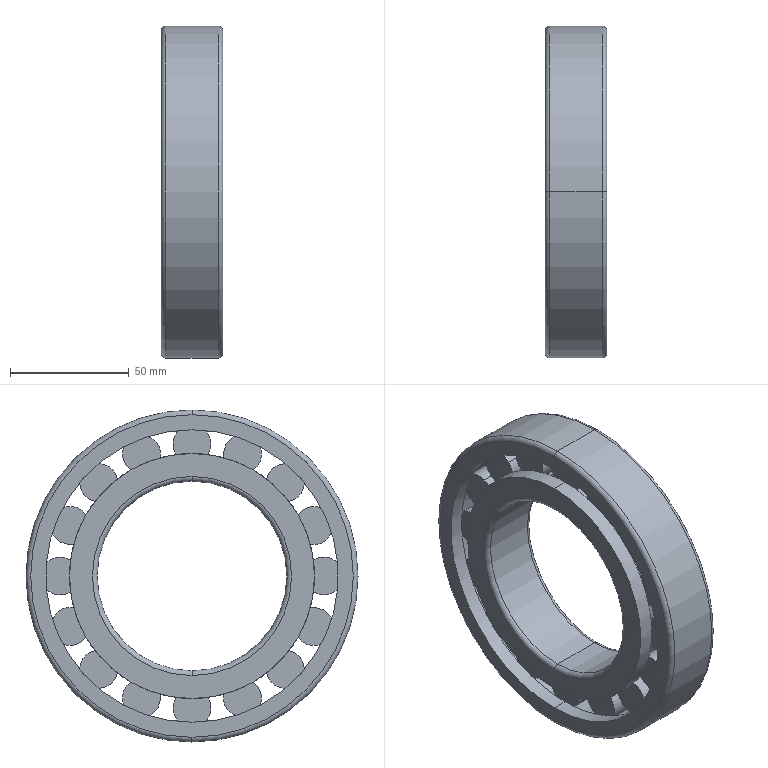Part | SolidWorks | features Revolution 3, CirPattern 1 | 1 solid | 200 faces | box 26 x 140 x 140 mm | volume 191182 mm3 | plane 100 | cylinder 92 | torus 8 | commonest cylinder face diameters 16 x48 95.3 x16 127.3 x16 103.3 x4 123.3 x4 80 x2